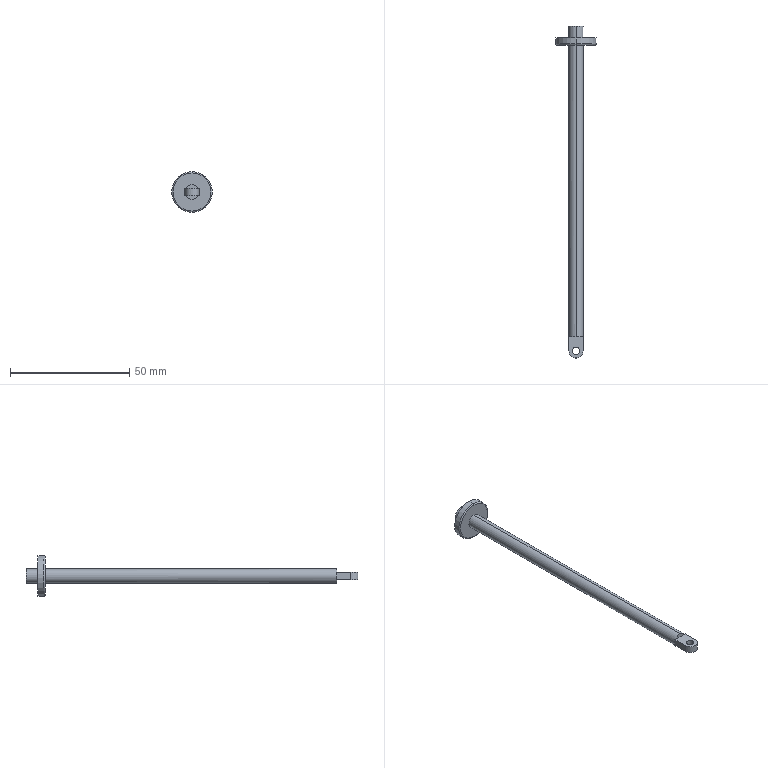Part | SolidWorks | features ICE 2, Extrusion 1, Fillet 1 | 1 solid | 24 faces | box 17 x 139 x 17 mm | volume 4398 mm3 | plane 13 | cylinder 9 | torus 2 | commonest cylinder face diameters 6 x5 3 x2 17 x2
STEP:
#1=CARTESIAN_POINT('',(0.,122.,-8.));
#2=VERTEX_POINT('',#1);
#3=CARTESIAN_POINT('',(0.,122.,8.));
#4=VERTEX_POINT('',#3);
#5=CARTESIAN_POINT('',(0.,122.,0.));
#6=DIRECTION('',(0.,-1.,0.));
#7=DIRECTION('',(0.,0.,1.));
#8=AXIS2_PLACEMENT_3D('',#5,#6,#7);
#9=CIRCLE('',#8,8.);
#10=EDGE_CURVE('',#2,#4,#9,.T.);
#11=ORIENTED_EDGE('',*,*,#10,.F.);
#12=CARTESIAN_POINT('',(0.,122.5,-8.5));
#13=VERTEX_POINT('',#12);
#14=CARTESIAN_POINT('',(0.,122.5,-8.));
#15=DIRECTION('',(1.,0.,0.));
#16=DIRECTION('',(0.,0.,-1.));
#17=AXIS2_PLACEMENT_3D('',#14,#15,#16);
#18=CIRCLE('',#17,0.5);
#19=EDGE_CURVE('',#2,#13,#18,.T.);
#20=ORIENTED_EDGE('',*,*,#19,.T.);
#21=CARTESIAN_POINT('',(0.,122.5,8.5));
#22=VERTEX_POINT('',#21);
#23=CARTESIAN_POINT('',(0.,122.5,0.));
#24=DIRECTION('',(0.,1.,0.));
#25=DIRECTION('',(0.,0.,1.));
#26=AXIS2_PLACEMENT_3D('',#23,#24,#25);
#27=CIRCLE('',#26,8.5);
#28=EDGE_CURVE('',#22,#13,#27,.T.);
#29=ORIENTED_EDGE('',*,*,#28,.F.);
#30=CARTESIAN_POINT('',(0.,122.5,8.));
#31=DIRECTION('',(-1.,0.,0.));
#32=DIRECTION('',(0.,0.,1.));
#33=AXIS2_PLACEMENT_3D('',#30,#31,#32);
#34=CIRCLE('',#33,0.5);
#35=EDGE_CURVE('',#4,#22,#34,.T.);
#36=ORIENTED_EDGE('',*,*,#35,.F.);
#37=EDGE_LOOP('',(#11,#20,#29,#36));
#38=FACE_OUTER_BOUND('',#37,.T.);
#39=CARTESIAN_POINT('',(0.,122.5,0.));
#40=DIRECTION('',(0.,1.,0.));
#41=DIRECTION('',(0.,0.,1.));
#42=AXIS2_PLACEMENT_3D('',#39,#40,#41);
#43=TOROIDAL_SURFACE('',#42,8.,0.5);
#44=ADVANCED_FACE('',(#38),#43,.T.);
#45=CARTESIAN_POINT('',(0.,130.,3.));
#46=VERTEX_POINT('',#45);
#47=CARTESIAN_POINT('',(0.,130.,-3.));
#48=VERTEX_POINT('',#47);
#49=CARTESIAN_POINT('',(0.,130.,0.));
#50=DIRECTION('',(0.,1.,0.));
#51=DIRECTION('',(0.,0.,1.));
#52=AXIS2_PLACEMENT_3D('',#49,#50,#51);
#53=CIRCLE('',#52,3.);
#54=EDGE_CURVE('',#46,#48,#53,.T.);
#55=ORIENTED_EDGE('',*,*,#54,.F.);
#56=CARTESIAN_POINT('',(0.,125.,3.));
#57=VERTEX_POINT('',#56);
#58=CARTESIAN_POINT('',(0.,130.,3.));
#59=DIRECTION('',(0.,-1.,0.));
#60=VECTOR('',#59,1000.);
#61=LINE('',#58,#60);
#62=EDGE_CURVE('',#46,#57,#61,.T.);
#63=ORIENTED_EDGE('',*,*,#62,.T.);
#64=CARTESIAN_POINT('',(0.,125.,-3.));
#65=VERTEX_POINT('',#64);
#66=CARTESIAN_POINT('',(0.,125.,0.));
#67=DIRECTION('',(0.,1.,0.));
#68=DIRECTION('',(0.,0.,1.));
#69=AXIS2_PLACEMENT_3D('',#66,#67,#68);
#70=CIRCLE('',#69,3.);
#71=EDGE_CURVE('',#57,#65,#70,.T.);
#72=ORIENTED_EDGE('',*,*,#71,.T.);
#73=CARTESIAN_POINT('',(0.,130.,-3.));
#74=DIRECTION('',(0.,-1.,0.));
#75=VECTOR('',#74,1000.);
#76=LINE('',#73,#75);
#77=EDGE_CURVE('',#48,#65,#76,.T.);
#78=ORIENTED_EDGE('',*,*,#77,.F.);
#79=EDGE_LOOP('',(#55,#63,#72,#78));
#80=FACE_OUTER_BOUND('',#79,.T.);
#81=CARTESIAN_POINT('',(0.,130.,0.));
#82=DIRECTION('',(0.,-1.,0.));
#83=DIRECTION('',(0.,0.,-1.));
#84=AXIS2_PLACEMENT_3D('',#81,#82,#83);
#85=CYLINDRICAL_SURFACE('',#84,3.);
#86=ADVANCED_FACE('',(#80),#85,.T.);
#87=CARTESIAN_POINT('',(0.,125.,8.5));
#88=VERTEX_POINT('',#87);
#89=CARTESIAN_POINT('',(0.,125.,-8.5));
#90=VERTEX_POINT('',#89);
#91=CARTESIAN_POINT('',(0.,125.,0.));
#92=DIRECTION('',(0.,1.,0.));
#93=DIRECTION('',(0.,0.,1.));
#94=AXIS2_PLACEMENT_3D('',#91,#92,#93);
#95=CIRCLE('',#94,8.5);
#96=EDGE_CURVE('',#88,#90,#95,.T.);
#97=ORIENTED_EDGE('',*,*,#96,.F.);
#98=CARTESIAN_POINT('',(0.,125.,8.5));
#99=DIRECTION('',(0.,-1.,0.));
#100=VECTOR('',#99,1000.);
#101=LINE('',#98,#100);
#102=EDGE_CURVE('',#88,#22,#101,.T.);
#103=ORIENTED_EDGE('',*,*,#102,.T.);
#104=ORIENTED_EDGE('',*,*,#28,.T.);
#105=CARTESIAN_POINT('',(0.,125.,-8.5));
#106=DIRECTION('',(0.,-1.,0.));
#107=VECTOR('',#106,1000.);
#108=LINE('',#105,#107);
#109=EDGE_CURVE('',#90,#13,#108,.T.);
#110=ORIENTED_EDGE('',*,*,#109,.F.);
#111=EDGE_LOOP('',(#97,#103,#104,#110));
#112=FACE_OUTER_BOUND('',#111,.T.);
#113=CARTESIAN_POINT('',(0.,125.,0.));
#114=DIRECTION('',(0.,-1.,0.));
#115=DIRECTION('',(0.,0.,-1.));
#116=AXIS2_PLACEMENT_3D('',#113,#114,#115);
#117=CYLINDRICAL_SURFACE('',#116,8.5);
#118=ADVANCED_FACE('',(#112),#117,.T.);
#119=CARTESIAN_POINT('',(-1.5,-6.,1.5));
#120=VERTEX_POINT('',#119);
#121=CARTESIAN_POINT('',(1.5,-6.,1.5));
#122=VERTEX_POINT('',#121);
#123=CARTESIAN_POINT('',(0.,-6.,1.5));
#124=DIRECTION('',(0.,0.,1.));
#125=DIRECTION('',(1.,0.,0.));
#126=AXIS2_PLACEMENT_3D('',#123,#124,#125);
#127=CIRCLE('',#126,1.5);
#128=EDGE_CURVE('',#120,#122,#127,.T.);
#129=ORIENTED_EDGE('',*,*,#128,.T.);
#130=CARTESIAN_POINT('',(1.5,-6.,-1.5));
#131=VERTEX_POINT('',#130);
#132=CARTESIAN_POINT('',(1.5,-6.,1.5));
#133=DIRECTION('',(0.,0.,-1.));
#134=VECTOR('',#133,1000.);
#135=LINE('',#132,#134);
#136=EDGE_CURVE('',#122,#131,#135,.T.);
#137=ORIENTED_EDGE('',*,*,#136,.T.);
#138=CARTESIAN_POINT('',(-1.5,-6.,-1.5));
#139=VERTEX_POINT('',#138);
#140=CARTESIAN_POINT('',(0.,-6.,-1.5));
#141=DIRECTION('',(0.,0.,1.));
#142=DIRECTION('',(1.,0.,0.));
#143=AXIS2_PLACEMENT_3D('',#140,#141,#142);
#144=CIRCLE('',#143,1.5);
#145=EDGE_CURVE('',#139,#131,#144,.T.);
#146=ORIENTED_EDGE('',*,*,#145,.F.);
#147=CARTESIAN_POINT('',(-1.5,-6.,1.5));
#148=DIRECTION('',(0.,0.,-1.));
#149=VECTOR('',#148,1000.);
#150=LINE('',#147,#149);
#151=EDGE_CURVE('',#120,#139,#150,.T.);
#152=ORIENTED_EDGE('',*,*,#151,.F.);
#153=EDGE_LOOP('',(#129,#137,#146,#152));
#154=FACE_OUTER_BOUND('',#153,.T.);
#155=CARTESIAN_POINT('',(0.,-6.,1.5));
#156=DIRECTION('',(0.,0.,-1.));
#157=DIRECTION('',(-1.,0.,0.));
#158=AXIS2_PLACEMENT_3D('',#155,#156,#157);
#159=CYLINDRICAL_SURFACE('',#158,1.5);
#160=ADVANCED_FACE('',(#154),#159,.F.);
#161=CARTESIAN_POINT('',(0.,122.,3.));
#162=VERTEX_POINT('',#161);
#163=CARTESIAN_POINT('',(0.,122.,-3.));
#164=VERTEX_POINT('',#163);
#165=CARTESIAN_POINT('',(0.,122.,0.));
#166=DIRECTION('',(0.,1.,0.));
#167=DIRECTION('',(0.,0.,1.));
#168=AXIS2_PLACEMENT_3D('',#165,#166,#167);
#169=CIRCLE('',#168,3.);
#170=EDGE_CURVE('',#162,#164,#169,.T.);
#171=ORIENTED_EDGE('',*,*,#170,.F.);
#172=CARTESIAN_POINT('',(0.,0.,3.));
#173=VERTEX_POINT('',#172);
#174=CARTESIAN_POINT('',(0.,130.,3.));
#175=DIRECTION('',(0.,-1.,0.));
#176=VECTOR('',#175,1000.);
#177=LINE('',#174,#176);
#178=EDGE_CURVE('',#162,#173,#177,.T.);
#179=ORIENTED_EDGE('',*,*,#178,.T.);
#180=CARTESIAN_POINT('',(2.598,0.,1.5));
#181=VERTEX_POINT('',#180);
#182=CARTESIAN_POINT('',(0.,0.,0.));
#183=DIRECTION('',(0.,1.,0.));
#184=DIRECTION('',(0.,0.,1.));
#185=AXIS2_PLACEMENT_3D('',#182,#183,#184);
#186=CIRCLE('',#185,3.);
#187=EDGE_CURVE('',#173,#181,#186,.T.);
#188=ORIENTED_EDGE('',*,*,#187,.T.);
#189=CARTESIAN_POINT('',(3.,0.,0.));
#190=VERTEX_POINT('',#189);
#191=CARTESIAN_POINT('',(0.,0.,0.));
#192=DIRECTION('',(0.,1.,0.));
#193=DIRECTION('',(0.,0.,1.));
#194=AXIS2_PLACEMENT_3D('',#191,#192,#193);
#195=CIRCLE('',#194,3.);
#196=EDGE_CURVE('',#181,#190,#195,.T.);
#197=ORIENTED_EDGE('',*,*,#196,.T.);
#198=CARTESIAN_POINT('',(2.598,0.,-1.5));
#199=VERTEX_POINT('',#198);
#200=CARTESIAN_POINT('',(0.,0.,0.));
#201=DIRECTION('',(0.,1.,0.));
#202=DIRECTION('',(0.,0.,1.));
#203=AXIS2_PLACEMENT_3D('',#200,#201,#202);
#204=CIRCLE('',#203,3.);
#205=EDGE_CURVE('',#190,#199,#204,.T.);
#206=ORIENTED_EDGE('',*,*,#205,.T.);
#207=CARTESIAN_POINT('',(0.,0.,-3.));
#208=VERTEX_POINT('',#207);
#209=CARTESIAN_POINT('',(0.,0.,0.));
#210=DIRECTION('',(0.,1.,0.));
#211=DIRECTION('',(0.,0.,1.));
#212=AXIS2_PLACEMENT_3D('',#209,#210,#211);
#213=CIRCLE('',#212,3.);
#214=EDGE_CURVE('',#199,#208,#213,.T.);
#215=ORIENTED_EDGE('',*,*,#214,.T.);
#216=CARTESIAN_POINT('',(0.,130.,-3.));
#217=DIRECTION('',(0.,-1.,0.));
#218=VECTOR('',#217,1000.);
#219=LINE('',#216,#218);
#220=EDGE_CURVE('',#164,#208,#219,.T.);
#221=ORIENTED_EDGE('',*,*,#220,.F.);
#222=EDGE_LOOP('',(#171,#179,#188,#197,#206,#215,#221));
#223=FACE_OUTER_BOUND('',#222,.T.);
#224=CARTESIAN_POINT('',(0.,130.,0.));
#225=DIRECTION('',(0.,-1.,0.));
#226=DIRECTION('',(0.,0.,-1.));
#227=AXIS2_PLACEMENT_3D('',#224,#225,#226);
#228=CYLINDRICAL_SURFACE('',#227,3.);
#229=ADVANCED_FACE('',(#223),#228,.T.);
#230=ORIENTED_EDGE('',*,*,#178,.F.);
#231=CARTESIAN_POINT('',(0.,122.,0.));
#232=DIRECTION('',(0.,1.,0.));
#233=DIRECTION('',(0.,0.,1.));
#234=AXIS2_PLACEMENT_3D('',#231,#232,#233);
#235=CIRCLE('',#234,3.);
#236=EDGE_CURVE('',#164,#162,#235,.T.);
#237=ORIENTED_EDGE('',*,*,#236,.F.);
#238=ORIENTED_EDGE('',*,*,#220,.T.);
#239=CARTESIAN_POINT('',(-2.598,0.,-1.5));
#240=VERTEX_POINT('',#239);
#241=CARTESIAN_POINT('',(0.,0.,0.));
#242=DIRECTION('',(0.,1.,0.));
#243=DIRECTION('',(0.,0.,1.));
#244=AXIS2_PLACEMENT_3D('',#241,#242,#243);
#245=CIRCLE('',#244,3.);
#246=EDGE_CURVE('',#208,#240,#245,.T.);
#247=ORIENTED_EDGE('',*,*,#246,.T.);
#248=CARTESIAN_POINT('',(-3.,0.,0.));
#249=VERTEX_POINT('',#248);
#250=CARTESIAN_POINT('',(0.,0.,0.));
#251=DIRECTION('',(0.,1.,0.));
#252=DIRECTION('',(0.,0.,1.));
#253=AXIS2_PLACEMENT_3D('',#250,#251,#252);
#254=CIRCLE('',#253,3.);
#255=EDGE_CURVE('',#240,#249,#254,.T.);
#256=ORIENTED_EDGE('',*,*,#255,.T.);
#257=CARTESIAN_POINT('',(-2.598,0.,1.5));
#258=VERTEX_POINT('',#257);
#259=CARTESIAN_POINT('',(0.,0.,0.));
#260=DIRECTION('',(0.,1.,0.));
#261=DIRECTION('',(0.,0.,1.));
#262=AXIS2_PLACEMENT_3D('',#259,#260,#261);
#263=CIRCLE('',#262,3.);
#264=EDGE_CURVE('',#249,#258,#263,.T.);
#265=ORIENTED_EDGE('',*,*,#264,.T.);
#266=CARTESIAN_POINT('',(0.,0.,0.));
#267=DIRECTION('',(0.,1.,0.));
#268=DIRECTION('',(0.,0.,1.));
#269=AXIS2_PLACEMENT_3D('',#266,#267,#268);
#270=CIRCLE('',#269,3.);
#271=EDGE_CURVE('',#258,#173,#270,.T.);
#272=ORIENTED_EDGE('',*,*,#271,.T.);
#273=EDGE_LOOP('',(#230,#237,#238,#247,#256,#265,#272));
#274=FACE_OUTER_BOUND('',#273,.T.);
#275=CARTESIAN_POINT('',(0.,130.,0.));
#276=DIRECTION('',(0.,-1.,0.));
#277=DIRECTION('',(0.,0.,-1.));
#278=AXIS2_PLACEMENT_3D('',#275,#276,#277);
#279=CYLINDRICAL_SURFACE('',#278,3.);
#280=ADVANCED_FACE('',(#274),#279,.T.);
#281=CARTESIAN_POINT('',(0.,0.,-1.5));
#282=DIRECTION('',(1.,0.,0.));
#283=VECTOR('',#282,1000.);
#284=LINE('',#281,#283);
#285=EDGE_CURVE('',#240,#199,#284,.T.);
#286=ORIENTED_EDGE('',*,*,#285,.F.);
#287=ORIENTED_EDGE('',*,*,#246,.F.);
#288=ORIENTED_EDGE('',*,*,#214,.F.);
#289=EDGE_LOOP('',(#286,#287,#288));
#290=FACE_OUTER_BOUND('',#289,.T.);
#291=CARTESIAN_POINT('',(0.,0.,0.));
#292=DIRECTION('',(0.,1.,0.));
#293=DIRECTION('',(0.,0.,1.));
#294=AXIS2_PLACEMENT_3D('',#291,#292,#293);
#295=PLANE('',#294);
#296=ADVANCED_FACE('',(#290),#295,.F.);
#297=ORIENTED_EDGE('',*,*,#271,.F.);
#298=CARTESIAN_POINT('',(0.,0.,1.5));
#299=DIRECTION('',(1.,0.,0.));
#300=VECTOR('',#299,1000.);
#301=LINE('',#298,#300);
#302=EDGE_CURVE('',#258,#181,#301,.T.);
#303=ORIENTED_EDGE('',*,*,#302,.T.);
#304=ORIENTED_EDGE('',*,*,#187,.F.);
#305=EDGE_LOOP('',(#297,#303,#304));
#306=FACE_OUTER_BOUND('',#305,.T.);
#307=CARTESIAN_POINT('',(0.,0.,0.));
#308=DIRECTION('',(0.,1.,0.));
#309=DIRECTION('',(0.,0.,1.));
#310=AXIS2_PLACEMENT_3D('',#307,#308,#309);
#311=PLANE('',#310);
#312=ADVANCED_FACE('',(#306),#311,.F.);
#313=ORIENTED_EDGE('',*,*,#196,.F.);
#314=CARTESIAN_POINT('',(3.,0.,1.5));
#315=VERTEX_POINT('',#314);
#316=CARTESIAN_POINT('',(0.,0.,1.5));
#317=DIRECTION('',(1.,0.,0.));
#318=VECTOR('',#317,1000.);
#319=LINE('',#316,#318);
#320=EDGE_CURVE('',#181,#315,#319,.T.);
#321=ORIENTED_EDGE('',*,*,#320,.T.);
#322=CARTESIAN_POINT('',(3.,0.,1.5));
#323=DIRECTION('',(0.,0.,-1.));
#324=VECTOR('',#323,1000.);
#325=LINE('',#322,#324);
#326=EDGE_CURVE('',#315,#190,#325,.T.);
#327=ORIENTED_EDGE('',*,*,#326,.T.);
#328=EDGE_LOOP('',(#313,#321,#327));
#329=FACE_OUTER_BOUND('',#328,.T.);
#330=CARTESIAN_POINT('',(0.,0.,1.5));
#331=DIRECTION('',(0.,1.,0.));
#332=DIRECTION('',(0.,0.,1.));
#333=AXIS2_PLACEMENT_3D('',#330,#331,#332);
#334=PLANE('',#333);
#335=ADVANCED_FACE('',(#329),#334,.T.);
#336=ORIENTED_EDGE('',*,*,#205,.F.);
#337=CARTESIAN_POINT('',(3.,0.,-1.5));
#338=VERTEX_POINT('',#337);
#339=CARTESIAN_POINT('',(3.,0.,1.5));
#340=DIRECTION('',(0.,0.,-1.));
#341=VECTOR('',#340,1000.);
#342=LINE('',#339,#341);
#343=EDGE_CURVE('',#190,#338,#342,.T.);
#344=ORIENTED_EDGE('',*,*,#343,.T.);
#345=CARTESIAN_POINT('',(0.,0.,-1.5));
#346=DIRECTION('',(1.,0.,0.));
#347=VECTOR('',#346,1000.);
#348=LINE('',#345,#347);
#349=EDGE_CURVE('',#199,#338,#348,.T.);
#350=ORIENTED_EDGE('',*,*,#349,.F.);
#351=EDGE_LOOP('',(#336,#344,#350));
#352=FACE_OUTER_BOUND('',#351,.T.);
#353=CARTESIAN_POINT('',(0.,0.,1.5));
#354=DIRECTION('',(0.,1.,0.));
#355=DIRECTION('',(0.,0.,1.));
#356=AXIS2_PLACEMENT_3D('',#353,#354,#355);
#357=PLANE('',#356);
#358=ADVANCED_FACE('',(#352),#357,.T.);
#359=ORIENTED_EDGE('',*,*,#255,.F.);
#360=CARTESIAN_POINT('',(-3.,0.,-1.5));
#361=VERTEX_POINT('',#360);
#362=CARTESIAN_POINT('',(0.,0.,-1.5));
#363=DIRECTION('',(1.,0.,0.));
#364=VECTOR('',#363,1000.);
#365=LINE('',#362,#364);
#366=EDGE_CURVE('',#361,#240,#365,.T.);
#367=ORIENTED_EDGE('',*,*,#366,.F.);
#368=CARTESIAN_POINT('',(-3.,0.,1.5));
#369=DIRECTION('',(0.,0.,-1.));
#370=VECTOR('',#369,1000.);
#371=LINE('',#368,#370);
#372=EDGE_CURVE('',#249,#361,#371,.T.);
#373=ORIENTED_EDGE('',*,*,#372,.F.);
#374=EDGE_LOOP('',(#359,#367,#373));
#375=FACE_OUTER_BOUND('',#374,.T.);
#376=CARTESIAN_POINT('',(0.,0.,1.5));
#377=DIRECTION('',(0.,1.,0.));
#378=DIRECTION('',(0.,0.,1.));
#379=AXIS2_PLACEMENT_3D('',#376,#377,#378);
#380=PLANE('',#379);
#381=ADVANCED_FACE('',(#375),#380,.T.);
#382=ORIENTED_EDGE('',*,*,#264,.F.);
#383=CARTESIAN_POINT('',(-3.,0.,1.5));
#384=VERTEX_POINT('',#383);
#385=CARTESIAN_POINT('',(-3.,0.,1.5));
#386=DIRECTION('',(0.,0.,-1.));
#387=VECTOR('',#386,1000.);
#388=LINE('',#385,#387);
#389=EDGE_CURVE('',#384,#249,#388,.T.);
#390=ORIENTED_EDGE('',*,*,#389,.F.);
#391=CARTESIAN_POINT('',(0.,0.,1.5));
#392=DIRECTION('',(1.,0.,0.));
#393=VECTOR('',#392,1000.);
#394=LINE('',#391,#393);
#395=EDGE_CURVE('',#384,#258,#394,.T.);
#396=ORIENTED_EDGE('',*,*,#395,.T.);
#397=EDGE_LOOP('',(#382,#390,#396));
#398=FACE_OUTER_BOUND('',#397,.T.);
#399=CARTESIAN_POINT('',(0.,0.,1.5));
#400=DIRECTION('',(0.,1.,0.));
#401=DIRECTION('',(0.,0.,1.));
#402=AXIS2_PLACEMENT_3D('',#399,#400,#401);
#403=PLANE('',#402);
#404=ADVANCED_FACE('',(#398),#403,.T.);
#405=CARTESIAN_POINT('',(-3.,-6.,-1.5));
#406=VERTEX_POINT('',#405);
#407=CARTESIAN_POINT('',(-3.,0.,-1.5));
#408=DIRECTION('',(0.,-1.,0.));
#409=VECTOR('',#408,1000.);
#410=LINE('',#407,#409);
#411=EDGE_CURVE('',#361,#406,#410,.T.);
#412=ORIENTED_EDGE('',*,*,#411,.T.);
#413=CARTESIAN_POINT('',(-3.,-6.,1.5));
#414=VERTEX_POINT('',#413);
#415=CARTESIAN_POINT('',(-3.,-6.,1.5));
#416=DIRECTION('',(0.,0.,-1.));
#417=VECTOR('',#416,1000.);
#418=LINE('',#415,#417);
#419=EDGE_CURVE('',#414,#406,#418,.T.);
#420=ORIENTED_EDGE('',*,*,#419,.F.);
#421=CARTESIAN_POINT('',(-3.,0.,1.5));
#422=DIRECTION('',(0.,-1.,0.));
#423=VECTOR('',#422,1000.);
#424=LINE('',#421,#423);
#425=EDGE_CURVE('',#384,#414,#424,.T.);
#426=ORIENTED_EDGE('',*,*,#425,.F.);
#427=ORIENTED_EDGE('',*,*,#389,.T.);
#428=ORIENTED_EDGE('',*,*,#372,.T.);
#429=EDGE_LOOP('',(#412,#420,#426,#427,#428));
#430=FACE_OUTER_BOUND('',#429,.T.);
#431=CARTESIAN_POINT('',(-3.,0.,1.5));
#432=DIRECTION('',(1.,0.,0.));
#433=DIRECTION('',(0.,1.,0.));
#434=AXIS2_PLACEMENT_3D('',#431,#432,#433);
#435=PLANE('',#434);
#436=ADVANCED_FACE('',(#430),#435,.F.);
#437=CARTESIAN_POINT('',(3.,-6.,-1.5));
#438=VERTEX_POINT('',#437);
#439=CARTESIAN_POINT('',(0.,-6.,-1.5));
#440=DIRECTION('',(0.,0.,1.));
#441=DIRECTION('',(1.,0.,0.));
#442=AXIS2_PLACEMENT_3D('',#439,#440,#441);
#443=CIRCLE('',#442,3.);
#444=EDGE_CURVE('',#406,#438,#443,.T.);
#445=ORIENTED_EDGE('',*,*,#444,.T.);
#446=CARTESIAN_POINT('',(3.,-6.,1.5));
#447=VERTEX_POINT('',#446);
#448=CARTESIAN_POINT('',(3.,-6.,1.5));
#449=DIRECTION('',(0.,0.,-1.));
#450=VECTOR('',#449,1000.);
#451=LINE('',#448,#450);
#452=EDGE_CURVE('',#447,#438,#451,.T.);
#453=ORIENTED_EDGE('',*,*,#452,.F.);
#454=CARTESIAN_POINT('',(0.,-6.,1.5));
#455=DIRECTION('',(0.,0.,1.));
#456=DIRECTION('',(1.,0.,0.));
#457=AXIS2_PLACEMENT_3D('',#454,#455,#456);
#458=CIRCLE('',#457,3.);
#459=EDGE_CURVE('',#414,#447,#458,.T.);
#460=ORIENTED_EDGE('',*,*,#459,.F.);
#461=ORIENTED_EDGE('',*,*,#419,.T.);
#462=EDGE_LOOP('',(#445,#453,#460,#461));
#463=FACE_OUTER_BOUND('',#462,.T.);
#464=CARTESIAN_POINT('',(0.,-6.,1.5));
#465=DIRECTION('',(0.,0.,-1.));
#466=DIRECTION('',(-1.,0.,0.));
#467=AXIS2_PLACEMENT_3D('',#464,#465,#466);
#468=CYLINDRICAL_SURFACE('',#467,3.);
#469=ADVANCED_FACE('',(#463),#468,.T.);
#470=CARTESIAN_POINT('',(3.,0.,-1.5));
#471=DIRECTION('',(0.,-1.,0.));
#472=VECTOR('',#471,1000.);
#473=LINE('',#470,#472);
#474=EDGE_CURVE('',#338,#438,#473,.T.);
#475=ORIENTED_EDGE('',*,*,#474,.F.);
#476=ORIENTED_EDGE('',*,*,#343,.F.);
#477=ORIENTED_EDGE('',*,*,#326,.F.);
#478=CARTESIAN_POINT('',(3.,0.,1.5));
#479=DIRECTION('',(0.,-1.,0.));
#480=VECTOR('',#479,1000.);
#481=LINE('',#478,#480);
#482=EDGE_CURVE('',#315,#447,#481,.T.);
#483=ORIENTED_EDGE('',*,*,#482,.T.);
#484=ORIENTED_EDGE('',*,*,#452,.T.);
#485=EDGE_LOOP('',(#475,#476,#477,#483,#484));
#486=FACE_OUTER_BOUND('',#485,.T.);
#487=CARTESIAN_POINT('',(3.,0.,1.5));
#488=DIRECTION('',(1.,0.,0.));
#489=DIRECTION('',(0.,1.,0.));
#490=AXIS2_PLACEMENT_3D('',#487,#488,#489);
#491=PLANE('',#490);
#492=ADVANCED_FACE('',(#486),#491,.T.);
#493=ORIENTED_EDGE('',*,*,#136,.F.);
#494=CARTESIAN_POINT('',(0.,-6.,1.5));
#495=DIRECTION('',(0.,0.,1.));
#496=DIRECTION('',(1.,0.,0.));
#497=AXIS2_PLACEMENT_3D('',#494,#495,#496);
#498=CIRCLE('',#497,1.5);
#499=EDGE_CURVE('',#122,#120,#498,.T.);
#500=ORIENTED_EDGE('',*,*,#499,.T.);
#501=ORIENTED_EDGE('',*,*,#151,.T.);
#502=CARTESIAN_POINT('',(0.,-6.,-1.5));
#503=DIRECTION('',(0.,0.,1.));
#504=DIRECTION('',(1.,0.,0.));
#505=AXIS2_PLACEMENT_3D('',#502,#503,#504);
#506=CIRCLE('',#505,1.5);
#507=EDGE_CURVE('',#131,#139,#506,.T.);
#508=ORIENTED_EDGE('',*,*,#507,.F.);
#509=EDGE_LOOP('',(#493,#500,#501,#508));
#510=FACE_OUTER_BOUND('',#509,.T.);
#511=CARTESIAN_POINT('',(0.,-6.,1.5));
#512=DIRECTION('',(0.,0.,-1.));
#513=DIRECTION('',(-1.,0.,0.));
#514=AXIS2_PLACEMENT_3D('',#511,#512,#513);
#515=CYLINDRICAL_SURFACE('',#514,1.5);
#516=ADVANCED_FACE('',(#510),#515,.F.);
#517=ORIENTED_EDGE('',*,*,#425,.T.);
#518=ORIENTED_EDGE('',*,*,#459,.T.);
#519=ORIENTED_EDGE('',*,*,#482,.F.);
#520=ORIENTED_EDGE('',*,*,#320,.F.);
#521=ORIENTED_EDGE('',*,*,#302,.F.);
#522=ORIENTED_EDGE('',*,*,#395,.F.);
#523=EDGE_LOOP('',(#517,#518,#519,#520,#521,#522));
#524=FACE_OUTER_BOUND('',#523,.T.);
#525=ORIENTED_EDGE('',*,*,#128,.F.);
#526=ORIENTED_EDGE('',*,*,#499,.F.);
#527=EDGE_LOOP('',(#525,#526));
#528=FACE_BOUND('',#527,.T.);
#529=CARTESIAN_POINT('',(0.,0.,1.5));
#530=DIRECTION('',(0.,0.,1.));
#531=DIRECTION('',(1.,0.,0.));
#532=AXIS2_PLACEMENT_3D('',#529,#530,#531);
#533=PLANE('',#532);
#534=ADVANCED_FACE('',(#524,#528),#533,.T.);
#535=ORIENTED_EDGE('',*,*,#411,.F.);
#536=ORIENTED_EDGE('',*,*,#366,.T.);
#537=ORIENTED_EDGE('',*,*,#285,.T.);
#538=ORIENTED_EDGE('',*,*,#349,.T.);
#539=ORIENTED_EDGE('',*,*,#474,.T.);
#540=ORIENTED_EDGE('',*,*,#444,.F.);
#541=EDGE_LOOP('',(#535,#536,#537,#538,#539,#540));
#542=FACE_OUTER_BOUND('',#541,.T.);
#543=ORIENTED_EDGE('',*,*,#145,.T.);
#544=ORIENTED_EDGE('',*,*,#507,.T.);
#545=EDGE_LOOP('',(#543,#544));
#546=FACE_BOUND('',#545,.T.);
#547=CARTESIAN_POINT('',(0.,0.,-1.5));
#548=DIRECTION('',(0.,0.,1.));
#549=DIRECTION('',(1.,0.,0.));
#550=AXIS2_PLACEMENT_3D('',#547,#548,#549);
#551=PLANE('',#550);
#552=ADVANCED_FACE('',(#542,#546),#551,.F.);
#553=ORIENTED_EDGE('',*,*,#102,.F.);
#554=CARTESIAN_POINT('',(0.,125.,0.));
#555=DIRECTION('',(0.,1.,0.));
#556=DIRECTION('',(0.,0.,1.));
#557=AXIS2_PLACEMENT_3D('',#554,#555,#556);
#558=CIRCLE('',#557,8.5);
#559=EDGE_CURVE('',#90,#88,#558,.T.);
#560=ORIENTED_EDGE('',*,*,#559,.F.);
#561=ORIENTED_EDGE('',*,*,#109,.T.);
#562=CARTESIAN_POINT('',(0.,122.5,0.));
#563=DIRECTION('',(0.,1.,0.));
#564=DIRECTION('',(0.,0.,1.));
#565=AXIS2_PLACEMENT_3D('',#562,#563,#564);
#566=CIRCLE('',#565,8.5);
#567=EDGE_CURVE('',#13,#22,#566,.T.);
#568=ORIENTED_EDGE('',*,*,#567,.T.);
#569=EDGE_LOOP('',(#553,#560,#561,#568));
#570=FACE_OUTER_BOUND('',#569,.T.);
#571=CARTESIAN_POINT('',(0.,125.,0.));
#572=DIRECTION('',(0.,-1.,0.));
#573=DIRECTION('',(0.,0.,-1.));
#574=AXIS2_PLACEMENT_3D('',#571,#572,#573);
#575=CYLINDRICAL_SURFACE('',#574,8.5);
#576=ADVANCED_FACE('',(#570),#575,.T.);
#577=CARTESIAN_POINT('',(0.,125.,0.));
#578=DIRECTION('',(0.,1.,0.));
#579=DIRECTION('',(0.,0.,1.));
#580=AXIS2_PLACEMENT_3D('',#577,#578,#579);
#581=CIRCLE('',#580,3.);
#582=EDGE_CURVE('',#65,#57,#581,.T.);
#583=ORIENTED_EDGE('',*,*,#582,.F.);
#584=ORIENTED_EDGE('',*,*,#71,.F.);
#585=EDGE_LOOP('',(#583,#584));
#586=FACE_BOUND('',#585,.T.);
#587=ORIENTED_EDGE('',*,*,#559,.T.);
#588=ORIENTED_EDGE('',*,*,#96,.T.);
#589=EDGE_LOOP('',(#587,#588));
#590=FACE_OUTER_BOUND('',#589,.T.);
#591=CARTESIAN_POINT('',(0.,125.,0.));
#592=DIRECTION('',(0.,1.,0.));
#593=DIRECTION('',(0.,0.,1.));
#594=AXIS2_PLACEMENT_3D('',#591,#592,#593);
#595=PLANE('',#594);
#596=ADVANCED_FACE('',(#586,#590),#595,.T.);
#597=CARTESIAN_POINT('',(0.,122.,0.));
#598=DIRECTION('',(0.,-1.,0.));
#599=DIRECTION('',(0.,0.,1.));
#600=AXIS2_PLACEMENT_3D('',#597,#598,#599);
#601=CIRCLE('',#600,8.);
#602=EDGE_CURVE('',#4,#2,#601,.T.);
#603=ORIENTED_EDGE('',*,*,#602,.T.);
#604=ORIENTED_EDGE('',*,*,#10,.T.);
#605=EDGE_LOOP('',(#603,#604));
#606=FACE_OUTER_BOUND('',#605,.T.);
#607=ORIENTED_EDGE('',*,*,#236,.T.);
#608=ORIENTED_EDGE('',*,*,#170,.T.);
#609=EDGE_LOOP('',(#607,#608));
#610=FACE_BOUND('',#609,.T.);
#611=CARTESIAN_POINT('',(0.,122.,0.));
#612=DIRECTION('',(0.,1.,0.));
#613=DIRECTION('',(0.,0.,1.));
#614=AXIS2_PLACEMENT_3D('',#611,#612,#613);
#615=PLANE('',#614);
#616=ADVANCED_FACE('',(#606,#610),#615,.F.);
#617=CARTESIAN_POINT('',(0.,130.,0.));
#618=DIRECTION('',(0.,1.,0.));
#619=DIRECTION('',(0.,0.,1.));
#620=AXIS2_PLACEMENT_3D('',#617,#618,#619);
#621=CIRCLE('',#620,3.);
#622=EDGE_CURVE('',#48,#46,#621,.T.);
#623=ORIENTED_EDGE('',*,*,#622,.T.);
#624=ORIENTED_EDGE('',*,*,#54,.T.);
#625=EDGE_LOOP('',(#623,#624));
#626=FACE_OUTER_BOUND('',#625,.T.);
#627=CARTESIAN_POINT('',(0.,130.,0.));
#628=DIRECTION('',(0.,1.,0.));
#629=DIRECTION('',(0.,0.,1.));
#630=AXIS2_PLACEMENT_3D('',#627,#628,#629);
#631=PLANE('',#630);
#632=ADVANCED_FACE('',(#626),#631,.T.);
#633=ORIENTED_EDGE('',*,*,#62,.F.);
#634=ORIENTED_EDGE('',*,*,#622,.F.);
#635=ORIENTED_EDGE('',*,*,#77,.T.);
#636=ORIENTED_EDGE('',*,*,#582,.T.);
#637=EDGE_LOOP('',(#633,#634,#635,#636));
#638=FACE_OUTER_BOUND('',#637,.T.);
#639=CARTESIAN_POINT('',(0.,130.,0.));
#640=DIRECTION('',(0.,-1.,0.));
#641=DIRECTION('',(0.,0.,-1.));
#642=AXIS2_PLACEMENT_3D('',#639,#640,#641);
#643=CYLINDRICAL_SURFACE('',#642,3.);
#644=ADVANCED_FACE('',(#638),#643,.T.);
#645=ORIENTED_EDGE('',*,*,#19,.F.);
#646=ORIENTED_EDGE('',*,*,#602,.F.);
#647=ORIENTED_EDGE('',*,*,#35,.T.);
#648=ORIENTED_EDGE('',*,*,#567,.F.);
#649=EDGE_LOOP('',(#645,#646,#647,#648));
#650=FACE_OUTER_BOUND('',#649,.T.);
#651=CARTESIAN_POINT('',(0.,122.5,0.));
#652=DIRECTION('',(0.,1.,0.));
#653=DIRECTION('',(0.,0.,1.));
#654=AXIS2_PLACEMENT_3D('',#651,#652,#653);
#655=TOROIDAL_SURFACE('',#654,8.,0.5);
#656=ADVANCED_FACE('',(#650),#655,.T.);
#657=CLOSED_SHELL('',(#44,#86,#118,#160,#229,#280,#296,#312,#335,#358,#381,#404,#436,#469,#492,#516,#534,#552,#576,#596,#616,#632,#644,#656));
#658=MANIFOLD_SOLID_BREP('',#657);
#659=CARTESIAN_POINT('',(0.,0.,0.));
#660=DIRECTION('',(0.,0.,1.));
#661=DIRECTION('',(1.,0.,0.));
#662=AXIS2_PLACEMENT_3D('',#659,#660,#661);
#663=(LENGTH_UNIT()NAMED_UNIT(*)SI_UNIT(.MILLI.,.METRE.));
#664=UNCERTAINTY_MEASURE_WITH_UNIT(LENGTH_MEASURE(0.00001),#663,'','');
#665=(NAMED_UNIT(*)PLANE_ANGLE_UNIT()SI_UNIT($,.RADIAN.));
#666=(NAMED_UNIT(*)SI_UNIT($,.STERADIAN.)SOLID_ANGLE_UNIT());
#667=(GEOMETRIC_REPRESENTATION_CONTEXT(3)GLOBAL_UNCERTAINTY_ASSIGNED_CONTEXT((#664))GLOBAL_UNIT_ASSIGNED_CONTEXT((#663,#665,#666))REPRESENTATION_CONTEXT('',''));
#668=ADVANCED_BREP_SHAPE_REPRESENTATION('',(#658,#662),#667);